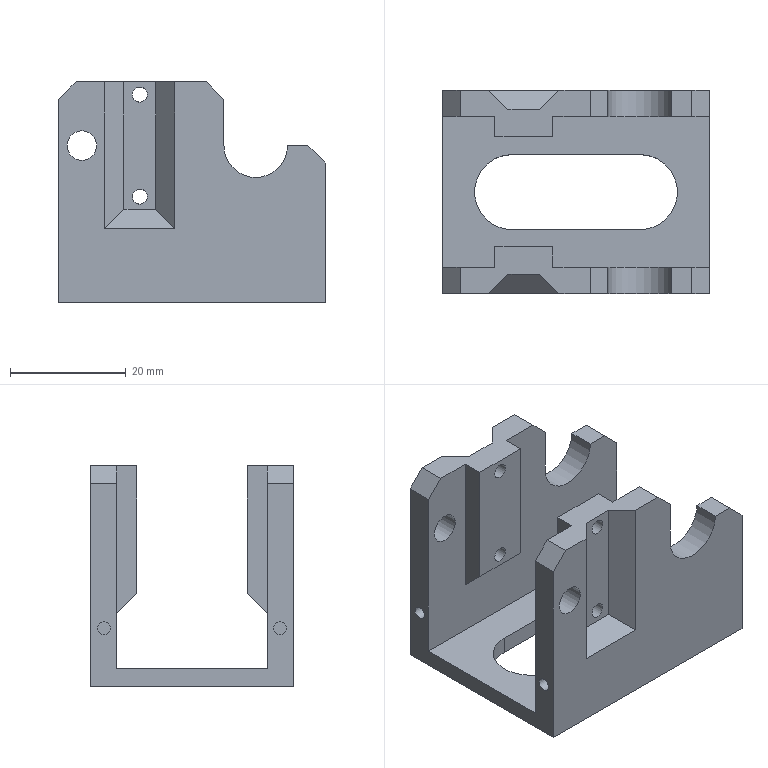Part | NX | features BREP 1 | 1 solid | 60 faces | box 46 x 35 x 38 mm | volume 15547 mm3 | plane 44 | cylinder 16 | commonest cylinder face diameters 2.2 x6 2.6 x4 5.1 x2 11 x2 13 x2